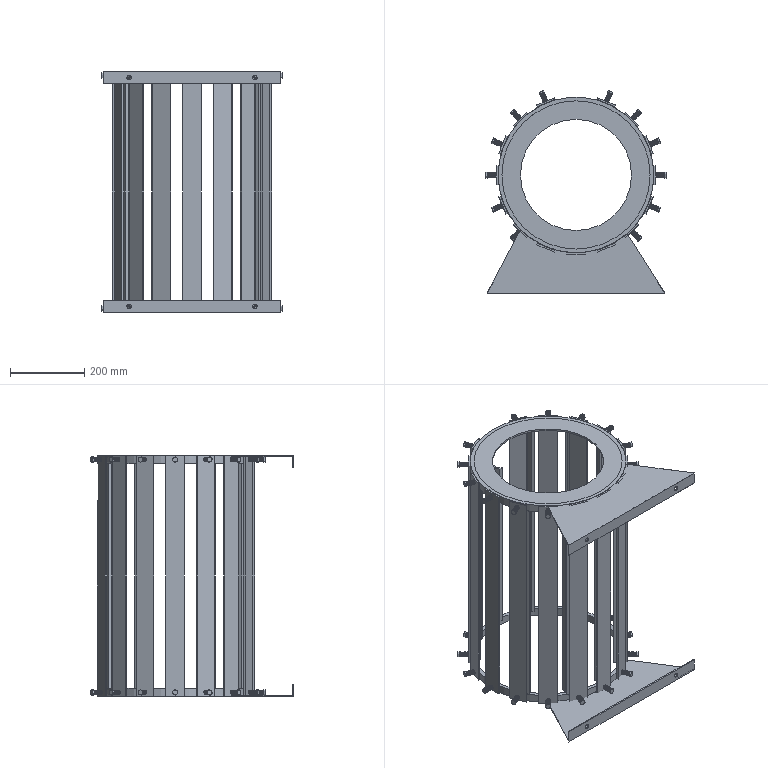Part | SolidWorks | features ReferencePattern 72, LocalCirPattern 2, MirrorCompFeat 1 | 104 solids | 1240 faces | box 488.345 x 547.074 x 650 mm | volume 5070939 mm3 | plane 590 | cone 300 | cylinder 230 | spline 120 | commonest cylinder face diameters 8 x184 400 x18 420 x18 12 x8 300 x2